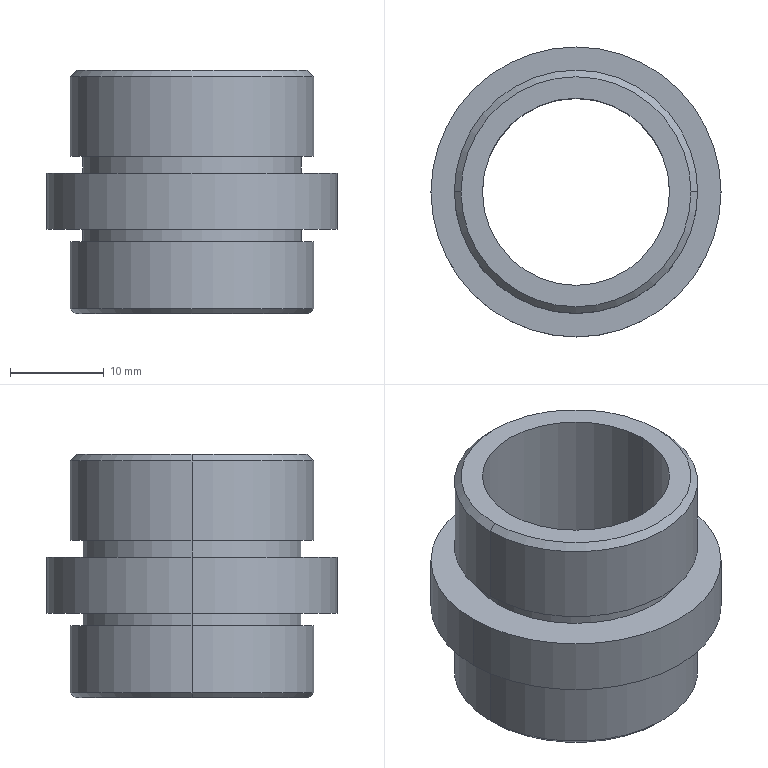Part | STEP file | 30 | 1 solid | 24 faces | box 31 x 31 x 26 mm | volume 6604 mm3 | cylinder 12 | cone 6 | plane 6 | commonest cylinder face diameters 23.4 x4 26 x4 20 x2 31 x2